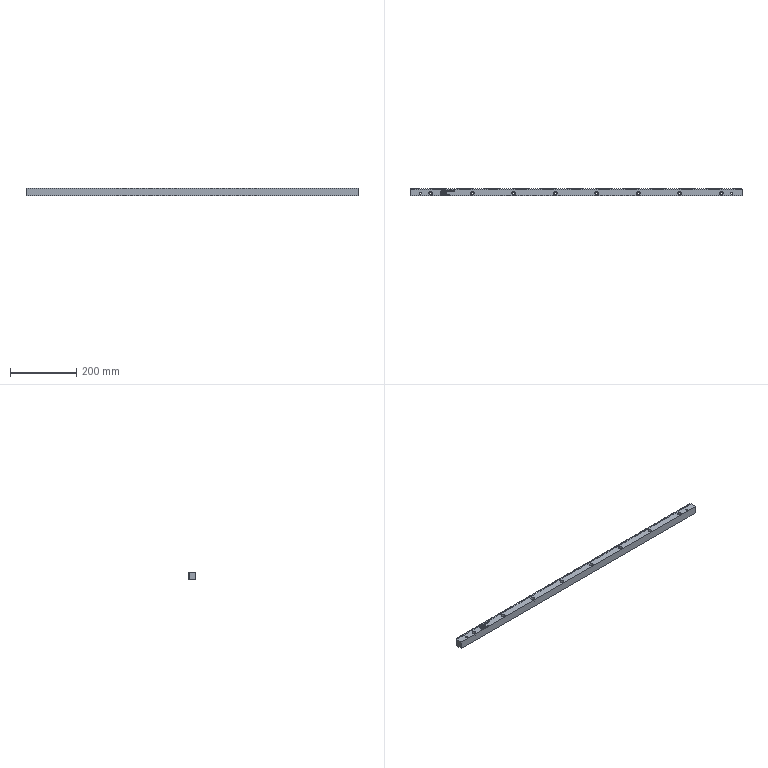Part | SolidWorks | features MBimport 1 | 1 solid | 2609 faces | box 1005 x 24 x 24 mm | volume 516028 mm3 | plane 2001 | spline 572 | cylinder 36 | commonest cylinder face diameters 7 x16 11 x16 5.7 x4